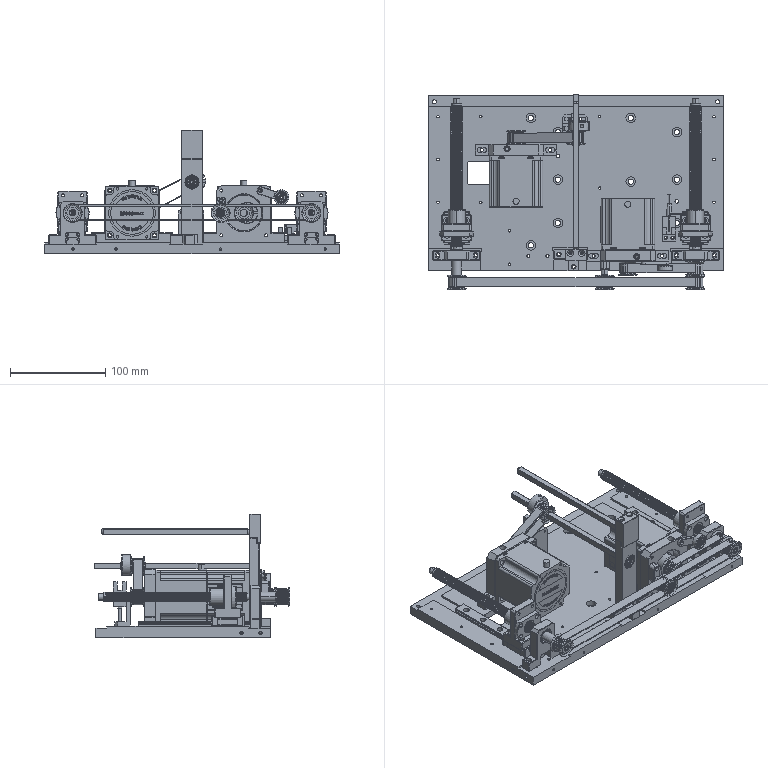Part | NX | features BREP 40 | 59 solids | 10961 faces | volume 1088437 mm3 | plane 6659 | cylinder 2560 | spline 860 | cone 378 | sphere 304 | torus 200 | commonest cylinder face diameters 0.46 x858 10 x336 15.66 x181 2.5 x108 3.3 x102 6 x78